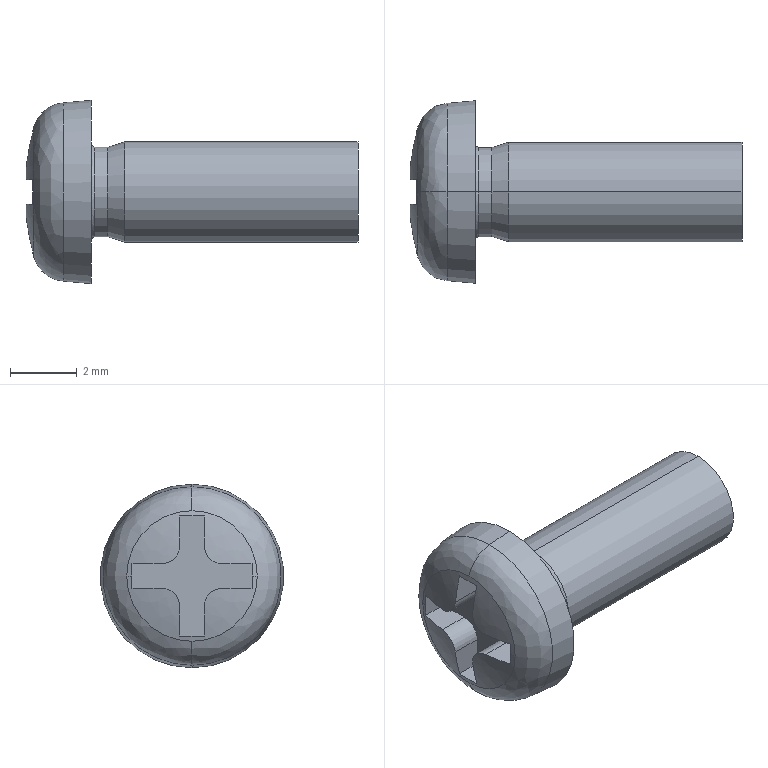Part | STEP file | 0243_316_NKJ3-8 | 1 solid | 33 faces | box 9.961 x 5.5 x 5.5 mm | volume 89.104 mm3 | plane 15 | cylinder 8 | spline 6 | cone 4 | commonest cylinder face diameters 1.1 x4 2.693 x2 3 x2